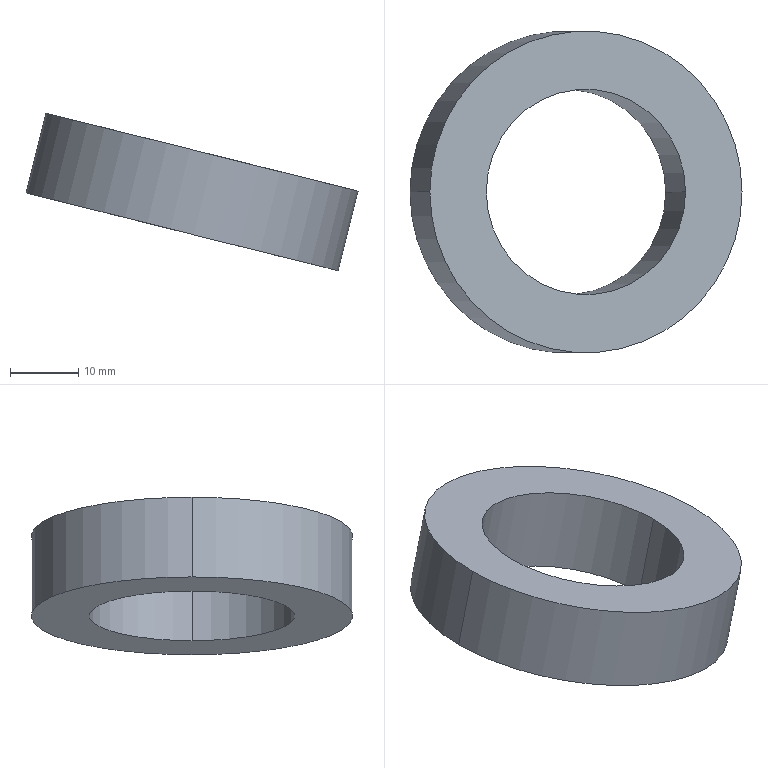Part | SolidWorks | features BaseBody 1 | 1 solid | 6 faces | box 48.507 x 47 x 23.012 mm | volume 12337 mm3 | cylinder 4 | plane 2 | commonest cylinder face diameters 30 x2 47 x2
STEP:
#1=CARTESIAN_POINT('',(-453.309,-4.,238.432));
#2=VERTEX_POINT('',#1);
#3=CARTESIAN_POINT('',(-482.418,-4.,245.688));
#4=VERTEX_POINT('',#3);
#5=CARTESIAN_POINT('',(-467.864,-4.,242.06));
#6=DIRECTION('',(-0.2419,0.,-0.9703));
#7=DIRECTION('',(0.9703,0.,-0.2419));
#8=AXIS2_PLACEMENT_3D('',#5,#6,#7);
#9=CIRCLE('',#8,15.);
#10=EDGE_CURVE('',#2,#4,#9,.T.);
#11=ORIENTED_EDGE('',*,*,#10,.F.);
#12=CARTESIAN_POINT('',(-456.212,-4.,226.788));
#13=VERTEX_POINT('',#12);
#14=CARTESIAN_POINT('',(-453.309,-4.,238.432));
#15=DIRECTION('',(-0.2419,0.,-0.9703));
#16=VECTOR('',#15,1000.);
#17=LINE('',#14,#16);
#18=EDGE_CURVE('',#2,#13,#17,.T.);
#19=ORIENTED_EDGE('',*,*,#18,.T.);
#20=CARTESIAN_POINT('',(-485.321,-4.,234.045));
#21=VERTEX_POINT('',#20);
#22=CARTESIAN_POINT('',(-470.766,-4.,230.417));
#23=DIRECTION('',(-0.2419,0.,-0.9703));
#24=DIRECTION('',(0.9703,0.,-0.2419));
#25=AXIS2_PLACEMENT_3D('',#22,#23,#24);
#26=CIRCLE('',#25,15.);
#27=EDGE_CURVE('',#13,#21,#26,.T.);
#28=ORIENTED_EDGE('',*,*,#27,.T.);
#29=CARTESIAN_POINT('',(-482.418,-4.,245.688));
#30=DIRECTION('',(-0.2419,0.,-0.9703));
#31=VECTOR('',#30,1000.);
#32=LINE('',#29,#31);
#33=EDGE_CURVE('',#4,#21,#32,.T.);
#34=ORIENTED_EDGE('',*,*,#33,.F.);
#35=EDGE_LOOP('',(#11,#19,#28,#34));
#36=FACE_OUTER_BOUND('',#35,.T.);
#37=CARTESIAN_POINT('',(-467.864,-4.,242.06));
#38=DIRECTION('',(-0.2419,0.,-0.9703));
#39=DIRECTION('',(-0.9703,0.,0.2419));
#40=AXIS2_PLACEMENT_3D('',#37,#38,#39);
#41=CYLINDRICAL_SURFACE('',#40,15.);
#42=ADVANCED_FACE('',(#36),#41,.F.);
#43=CARTESIAN_POINT('',(-490.666,-4.,247.744));
#44=VERTEX_POINT('',#43);
#45=CARTESIAN_POINT('',(-445.062,-4.,236.376));
#46=VERTEX_POINT('',#45);
#47=CARTESIAN_POINT('',(-467.864,-4.,242.06));
#48=DIRECTION('',(-0.2419,0.,-0.9703));
#49=DIRECTION('',(0.9703,0.,-0.2419));
#50=AXIS2_PLACEMENT_3D('',#47,#48,#49);
#51=CIRCLE('',#50,23.5);
#52=EDGE_CURVE('',#44,#46,#51,.T.);
#53=ORIENTED_EDGE('',*,*,#52,.T.);
#54=CARTESIAN_POINT('',(-447.964,-4.,224.732));
#55=VERTEX_POINT('',#54);
#56=CARTESIAN_POINT('',(-445.062,-4.,236.376));
#57=DIRECTION('',(-0.2419,0.,-0.9703));
#58=VECTOR('',#57,1000.);
#59=LINE('',#56,#58);
#60=EDGE_CURVE('',#46,#55,#59,.T.);
#61=ORIENTED_EDGE('',*,*,#60,.T.);
#62=CARTESIAN_POINT('',(-493.568,-4.,236.101));
#63=VERTEX_POINT('',#62);
#64=CARTESIAN_POINT('',(-470.766,-4.,230.417));
#65=DIRECTION('',(-0.2419,0.,-0.9703));
#66=DIRECTION('',(0.9703,0.,-0.2419));
#67=AXIS2_PLACEMENT_3D('',#64,#65,#66);
#68=CIRCLE('',#67,23.5);
#69=EDGE_CURVE('',#63,#55,#68,.T.);
#70=ORIENTED_EDGE('',*,*,#69,.F.);
#71=CARTESIAN_POINT('',(-490.666,-4.,247.744));
#72=DIRECTION('',(-0.2419,0.,-0.9703));
#73=VECTOR('',#72,1000.);
#74=LINE('',#71,#73);
#75=EDGE_CURVE('',#44,#63,#74,.T.);
#76=ORIENTED_EDGE('',*,*,#75,.F.);
#77=EDGE_LOOP('',(#53,#61,#70,#76));
#78=FACE_OUTER_BOUND('',#77,.T.);
#79=CARTESIAN_POINT('',(-467.864,-4.,242.06));
#80=DIRECTION('',(-0.2419,0.,-0.9703));
#81=DIRECTION('',(-0.9703,0.,0.2419));
#82=AXIS2_PLACEMENT_3D('',#79,#80,#81);
#83=CYLINDRICAL_SURFACE('',#82,23.5);
#84=ADVANCED_FACE('',(#78),#83,.T.);
#85=CARTESIAN_POINT('',(-470.766,-4.,230.417));
#86=DIRECTION('',(-0.2419,0.,-0.9703));
#87=DIRECTION('',(0.9703,0.,-0.2419));
#88=AXIS2_PLACEMENT_3D('',#85,#86,#87);
#89=CIRCLE('',#88,15.);
#90=EDGE_CURVE('',#21,#13,#89,.T.);
#91=ORIENTED_EDGE('',*,*,#90,.F.);
#92=ORIENTED_EDGE('',*,*,#27,.F.);
#93=EDGE_LOOP('',(#91,#92));
#94=FACE_BOUND('',#93,.T.);
#95=ORIENTED_EDGE('',*,*,#69,.T.);
#96=CARTESIAN_POINT('',(-470.766,-4.,230.417));
#97=DIRECTION('',(-0.2419,0.,-0.9703));
#98=DIRECTION('',(0.9703,0.,-0.2419));
#99=AXIS2_PLACEMENT_3D('',#96,#97,#98);
#100=CIRCLE('',#99,23.5);
#101=EDGE_CURVE('',#55,#63,#100,.T.);
#102=ORIENTED_EDGE('',*,*,#101,.T.);
#103=EDGE_LOOP('',(#95,#102));
#104=FACE_OUTER_BOUND('',#103,.T.);
#105=CARTESIAN_POINT('',(-470.766,-4.,230.417));
#106=DIRECTION('',(-0.2419,0.,-0.9703));
#107=DIRECTION('',(-0.9703,0.,0.2419));
#108=AXIS2_PLACEMENT_3D('',#105,#106,#107);
#109=PLANE('',#108);
#110=ADVANCED_FACE('',(#94,#104),#109,.T.);
#111=CARTESIAN_POINT('',(-467.864,-4.,242.06));
#112=DIRECTION('',(-0.2419,0.,-0.9703));
#113=DIRECTION('',(0.9703,0.,-0.2419));
#114=AXIS2_PLACEMENT_3D('',#111,#112,#113);
#115=CIRCLE('',#114,15.);
#116=EDGE_CURVE('',#4,#2,#115,.T.);
#117=ORIENTED_EDGE('',*,*,#116,.T.);
#118=ORIENTED_EDGE('',*,*,#10,.T.);
#119=EDGE_LOOP('',(#117,#118));
#120=FACE_BOUND('',#119,.T.);
#121=ORIENTED_EDGE('',*,*,#52,.F.);
#122=CARTESIAN_POINT('',(-467.864,-4.,242.06));
#123=DIRECTION('',(-0.2419,0.,-0.9703));
#124=DIRECTION('',(0.9703,0.,-0.2419));
#125=AXIS2_PLACEMENT_3D('',#122,#123,#124);
#126=CIRCLE('',#125,23.5);
#127=EDGE_CURVE('',#46,#44,#126,.T.);
#128=ORIENTED_EDGE('',*,*,#127,.F.);
#129=EDGE_LOOP('',(#121,#128));
#130=FACE_OUTER_BOUND('',#129,.T.);
#131=CARTESIAN_POINT('',(-467.864,-4.,242.06));
#132=DIRECTION('',(-0.2419,0.,-0.9703));
#133=DIRECTION('',(-0.9703,0.,0.2419));
#134=AXIS2_PLACEMENT_3D('',#131,#132,#133);
#135=PLANE('',#134);
#136=ADVANCED_FACE('',(#120,#130),#135,.F.);
#137=ORIENTED_EDGE('',*,*,#60,.F.);
#138=ORIENTED_EDGE('',*,*,#127,.T.);
#139=ORIENTED_EDGE('',*,*,#75,.T.);
#140=ORIENTED_EDGE('',*,*,#101,.F.);
#141=EDGE_LOOP('',(#137,#138,#139,#140));
#142=FACE_OUTER_BOUND('',#141,.T.);
#143=CARTESIAN_POINT('',(-467.864,-4.,242.06));
#144=DIRECTION('',(-0.2419,0.,-0.9703));
#145=DIRECTION('',(-0.9703,0.,0.2419));
#146=AXIS2_PLACEMENT_3D('',#143,#144,#145);
#147=CYLINDRICAL_SURFACE('',#146,23.5);
#148=ADVANCED_FACE('',(#142),#147,.T.);
#149=ORIENTED_EDGE('',*,*,#18,.F.);
#150=ORIENTED_EDGE('',*,*,#116,.F.);
#151=ORIENTED_EDGE('',*,*,#33,.T.);
#152=ORIENTED_EDGE('',*,*,#90,.T.);
#153=EDGE_LOOP('',(#149,#150,#151,#152));
#154=FACE_OUTER_BOUND('',#153,.T.);
#155=CARTESIAN_POINT('',(-467.864,-4.,242.06));
#156=DIRECTION('',(-0.2419,0.,-0.9703));
#157=DIRECTION('',(-0.9703,0.,0.2419));
#158=AXIS2_PLACEMENT_3D('',#155,#156,#157);
#159=CYLINDRICAL_SURFACE('',#158,15.);
#160=ADVANCED_FACE('',(#154),#159,.F.);
#161=CLOSED_SHELL('',(#42,#84,#110,#136,#148,#160));
#162=MANIFOLD_SOLID_BREP('',#161);
#163=CARTESIAN_POINT('',(0.,0.,0.));
#164=DIRECTION('',(0.,0.,1.));
#165=DIRECTION('',(1.,0.,0.));
#166=AXIS2_PLACEMENT_3D('',#163,#164,#165);
#167=(LENGTH_UNIT()NAMED_UNIT(*)SI_UNIT(.MILLI.,.METRE.));
#168=UNCERTAINTY_MEASURE_WITH_UNIT(LENGTH_MEASURE(0.00001),#167,'','');
#169=(NAMED_UNIT(*)PLANE_ANGLE_UNIT()SI_UNIT($,.RADIAN.));
#170=(NAMED_UNIT(*)SI_UNIT($,.STERADIAN.)SOLID_ANGLE_UNIT());
#171=(GEOMETRIC_REPRESENTATION_CONTEXT(3)GLOBAL_UNCERTAINTY_ASSIGNED_CONTEXT((#168))GLOBAL_UNIT_ASSIGNED_CONTEXT((#167,#169,#170))REPRESENTATION_CONTEXT('',''));
#172=ADVANCED_BREP_SHAPE_REPRESENTATION('',(#162,#166),#171);